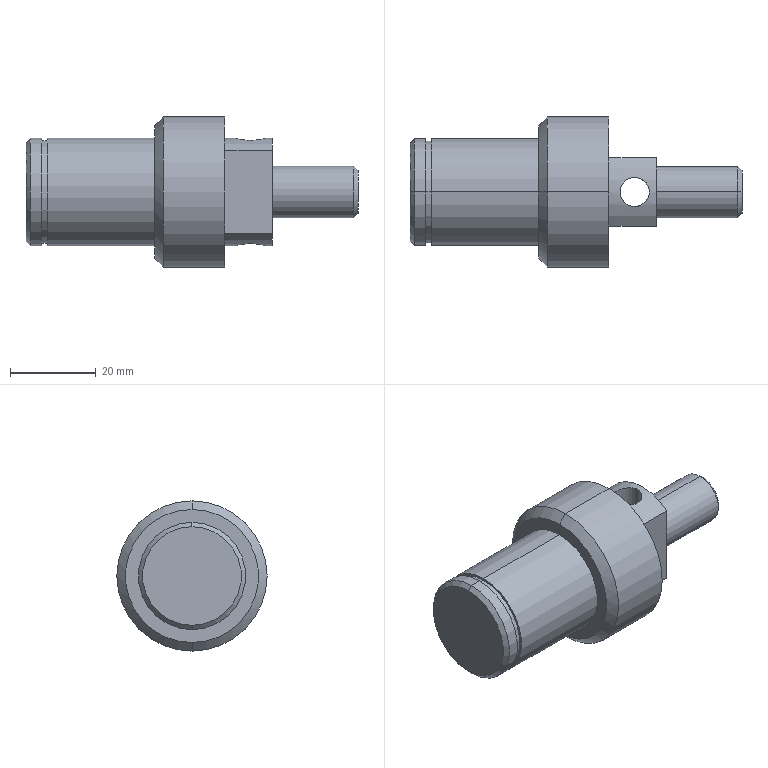Part | STEP file | 0228_214_Shaft | 1 solid | 30 faces | box 77.35 x 35 x 35 mm | volume 35572 mm3 | cylinder 15 | plane 9 | cone 6 | commonest cylinder face diameters 25 x7 6.8 x2 12 x2 23.9 x2 35 x2